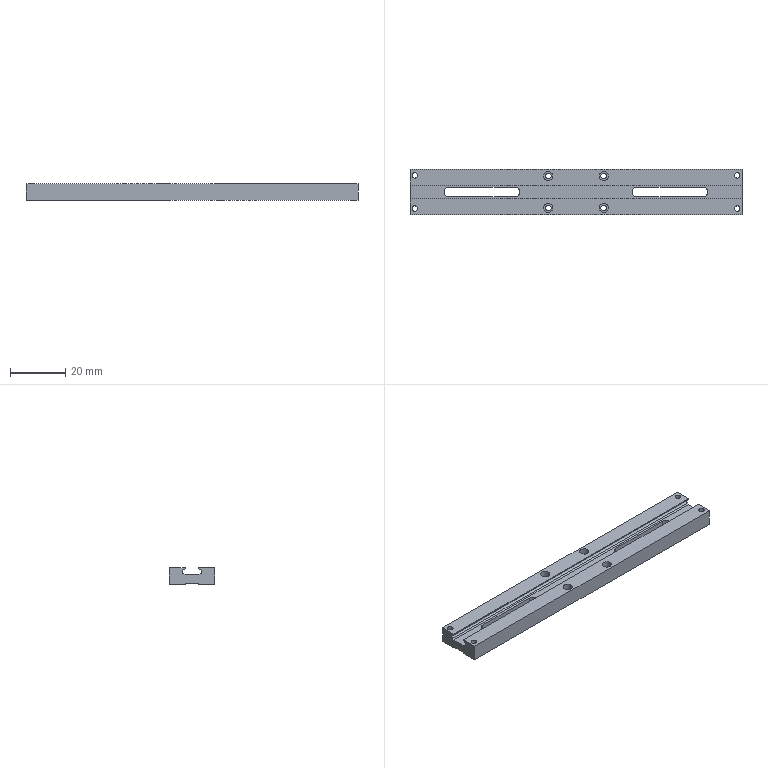Part | SolidWorks | features ICE 4, Cut 2, Extrusion 1 | 1 solid | 60 faces | box 120 x 16.4 x 6 mm | volume 8918 mm3 | cylinder 34 | plane 26 | commonest cylinder face diameters 2 x16 3.3 x8 3.4 x6 1.5 x4